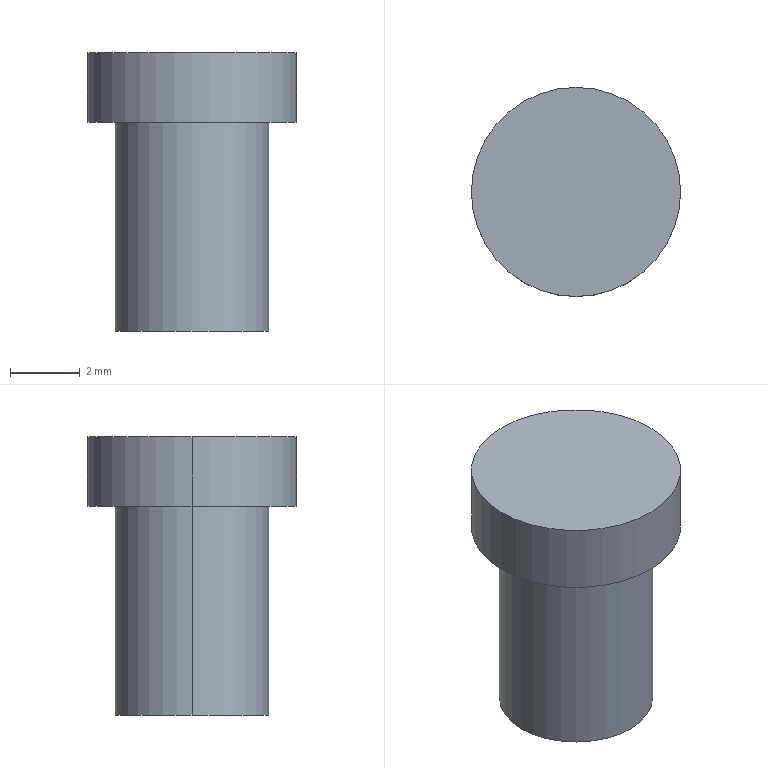Part | SolidWorks | features Extrusion 1, ICE 1 | 1 solid | 7 faces | box 6 x 6 x 8 mm | volume 147.781 mm3 | cylinder 4 | plane 3 | commonest cylinder face diameters 4.4 x2 6 x2
STEP:
#1=CARTESIAN_POINT('',(3.,0.,2.));
#2=VERTEX_POINT('',#1);
#3=CARTESIAN_POINT('',(-3.,0.,2.));
#4=VERTEX_POINT('',#3);
#5=CARTESIAN_POINT('',(0.,0.,2.));
#6=DIRECTION('',(0.,0.,1.));
#7=DIRECTION('',(1.,0.,0.));
#8=AXIS2_PLACEMENT_3D('',#5,#6,#7);
#9=CIRCLE('',#8,3.);
#10=EDGE_CURVE('',#2,#4,#9,.T.);
#11=ORIENTED_EDGE('',*,*,#10,.F.);
#12=CARTESIAN_POINT('',(3.,0.,0.));
#13=VERTEX_POINT('',#12);
#14=CARTESIAN_POINT('',(3.,0.,2.));
#15=DIRECTION('',(0.,0.,-1.));
#16=VECTOR('',#15,1000.);
#17=LINE('',#14,#16);
#18=EDGE_CURVE('',#2,#13,#17,.T.);
#19=ORIENTED_EDGE('',*,*,#18,.T.);
#20=CARTESIAN_POINT('',(-3.,0.,0.));
#21=VERTEX_POINT('',#20);
#22=CARTESIAN_POINT('',(0.,0.,0.));
#23=DIRECTION('',(0.,0.,1.));
#24=DIRECTION('',(1.,0.,0.));
#25=AXIS2_PLACEMENT_3D('',#22,#23,#24);
#26=CIRCLE('',#25,3.);
#27=EDGE_CURVE('',#13,#21,#26,.T.);
#28=ORIENTED_EDGE('',*,*,#27,.T.);
#29=CARTESIAN_POINT('',(-3.,0.,2.));
#30=DIRECTION('',(0.,0.,-1.));
#31=VECTOR('',#30,1000.);
#32=LINE('',#29,#31);
#33=EDGE_CURVE('',#4,#21,#32,.T.);
#34=ORIENTED_EDGE('',*,*,#33,.F.);
#35=EDGE_LOOP('',(#11,#19,#28,#34));
#36=FACE_OUTER_BOUND('',#35,.T.);
#37=CARTESIAN_POINT('',(0.,0.,2.));
#38=DIRECTION('',(0.,0.,-1.));
#39=DIRECTION('',(-1.,0.,0.));
#40=AXIS2_PLACEMENT_3D('',#37,#38,#39);
#41=CYLINDRICAL_SURFACE('',#40,3.);
#42=ADVANCED_FACE('',(#36),#41,.T.);
#43=CARTESIAN_POINT('',(2.2,0.,-6.));
#44=VERTEX_POINT('',#43);
#45=CARTESIAN_POINT('',(-2.2,0.,-6.));
#46=VERTEX_POINT('',#45);
#47=CARTESIAN_POINT('',(0.,0.,-6.));
#48=DIRECTION('',(0.,0.,1.));
#49=DIRECTION('',(1.,0.,0.));
#50=AXIS2_PLACEMENT_3D('',#47,#48,#49);
#51=CIRCLE('',#50,2.2);
#52=EDGE_CURVE('',#44,#46,#51,.T.);
#53=ORIENTED_EDGE('',*,*,#52,.T.);
#54=CARTESIAN_POINT('',(-2.2,0.,0.));
#55=VERTEX_POINT('',#54);
#56=CARTESIAN_POINT('',(-2.2,0.,-6.));
#57=DIRECTION('',(0.,0.,1.));
#58=VECTOR('',#57,1000.);
#59=LINE('',#56,#58);
#60=EDGE_CURVE('',#46,#55,#59,.T.);
#61=ORIENTED_EDGE('',*,*,#60,.T.);
#62=CARTESIAN_POINT('',(2.2,0.,0.));
#63=VERTEX_POINT('',#62);
#64=CARTESIAN_POINT('',(0.,0.,0.));
#65=DIRECTION('',(0.,0.,1.));
#66=DIRECTION('',(1.,0.,0.));
#67=AXIS2_PLACEMENT_3D('',#64,#65,#66);
#68=CIRCLE('',#67,2.2);
#69=EDGE_CURVE('',#63,#55,#68,.T.);
#70=ORIENTED_EDGE('',*,*,#69,.F.);
#71=CARTESIAN_POINT('',(2.2,0.,-6.));
#72=DIRECTION('',(0.,0.,1.));
#73=VECTOR('',#72,1000.);
#74=LINE('',#71,#73);
#75=EDGE_CURVE('',#44,#63,#74,.T.);
#76=ORIENTED_EDGE('',*,*,#75,.F.);
#77=EDGE_LOOP('',(#53,#61,#70,#76));
#78=FACE_OUTER_BOUND('',#77,.T.);
#79=CARTESIAN_POINT('',(0.,0.,-6.));
#80=DIRECTION('',(0.,0.,1.));
#81=DIRECTION('',(1.,0.,0.));
#82=AXIS2_PLACEMENT_3D('',#79,#80,#81);
#83=CYLINDRICAL_SURFACE('',#82,2.2);
#84=ADVANCED_FACE('',(#78),#83,.T.);
#85=ORIENTED_EDGE('',*,*,#60,.F.);
#86=CARTESIAN_POINT('',(0.,0.,-6.));
#87=DIRECTION('',(0.,0.,1.));
#88=DIRECTION('',(1.,0.,0.));
#89=AXIS2_PLACEMENT_3D('',#86,#87,#88);
#90=CIRCLE('',#89,2.2);
#91=EDGE_CURVE('',#46,#44,#90,.T.);
#92=ORIENTED_EDGE('',*,*,#91,.T.);
#93=ORIENTED_EDGE('',*,*,#75,.T.);
#94=CARTESIAN_POINT('',(0.,0.,0.));
#95=DIRECTION('',(0.,0.,1.));
#96=DIRECTION('',(1.,0.,0.));
#97=AXIS2_PLACEMENT_3D('',#94,#95,#96);
#98=CIRCLE('',#97,2.2);
#99=EDGE_CURVE('',#55,#63,#98,.T.);
#100=ORIENTED_EDGE('',*,*,#99,.F.);
#101=EDGE_LOOP('',(#85,#92,#93,#100));
#102=FACE_OUTER_BOUND('',#101,.T.);
#103=CARTESIAN_POINT('',(0.,0.,-6.));
#104=DIRECTION('',(0.,0.,1.));
#105=DIRECTION('',(1.,0.,0.));
#106=AXIS2_PLACEMENT_3D('',#103,#104,#105);
#107=CYLINDRICAL_SURFACE('',#106,2.2);
#108=ADVANCED_FACE('',(#102),#107,.T.);
#109=ORIENTED_EDGE('',*,*,#52,.F.);
#110=ORIENTED_EDGE('',*,*,#91,.F.);
#111=EDGE_LOOP('',(#109,#110));
#112=FACE_OUTER_BOUND('',#111,.T.);
#113=CARTESIAN_POINT('',(0.,0.,-6.));
#114=DIRECTION('',(0.,0.,1.));
#115=DIRECTION('',(1.,0.,0.));
#116=AXIS2_PLACEMENT_3D('',#113,#114,#115);
#117=PLANE('',#116);
#118=ADVANCED_FACE('',(#112),#117,.F.);
#119=ORIENTED_EDGE('',*,*,#18,.F.);
#120=CARTESIAN_POINT('',(0.,0.,2.));
#121=DIRECTION('',(0.,0.,1.));
#122=DIRECTION('',(1.,0.,0.));
#123=AXIS2_PLACEMENT_3D('',#120,#121,#122);
#124=CIRCLE('',#123,3.);
#125=EDGE_CURVE('',#4,#2,#124,.T.);
#126=ORIENTED_EDGE('',*,*,#125,.F.);
#127=ORIENTED_EDGE('',*,*,#33,.T.);
#128=CARTESIAN_POINT('',(0.,0.,0.));
#129=DIRECTION('',(0.,0.,1.));
#130=DIRECTION('',(1.,0.,0.));
#131=AXIS2_PLACEMENT_3D('',#128,#129,#130);
#132=CIRCLE('',#131,3.);
#133=EDGE_CURVE('',#21,#13,#132,.T.);
#134=ORIENTED_EDGE('',*,*,#133,.T.);
#135=EDGE_LOOP('',(#119,#126,#127,#134));
#136=FACE_OUTER_BOUND('',#135,.T.);
#137=CARTESIAN_POINT('',(0.,0.,2.));
#138=DIRECTION('',(0.,0.,-1.));
#139=DIRECTION('',(-1.,0.,0.));
#140=AXIS2_PLACEMENT_3D('',#137,#138,#139);
#141=CYLINDRICAL_SURFACE('',#140,3.);
#142=ADVANCED_FACE('',(#136),#141,.T.);
#143=ORIENTED_EDGE('',*,*,#125,.T.);
#144=ORIENTED_EDGE('',*,*,#10,.T.);
#145=EDGE_LOOP('',(#143,#144));
#146=FACE_OUTER_BOUND('',#145,.T.);
#147=CARTESIAN_POINT('',(0.,0.,2.));
#148=DIRECTION('',(0.,0.,1.));
#149=DIRECTION('',(1.,0.,0.));
#150=AXIS2_PLACEMENT_3D('',#147,#148,#149);
#151=PLANE('',#150);
#152=ADVANCED_FACE('',(#146),#151,.T.);
#153=ORIENTED_EDGE('',*,*,#69,.T.);
#154=ORIENTED_EDGE('',*,*,#99,.T.);
#155=EDGE_LOOP('',(#153,#154));
#156=FACE_BOUND('',#155,.T.);
#157=ORIENTED_EDGE('',*,*,#133,.F.);
#158=ORIENTED_EDGE('',*,*,#27,.F.);
#159=EDGE_LOOP('',(#157,#158));
#160=FACE_OUTER_BOUND('',#159,.T.);
#161=CARTESIAN_POINT('',(0.,0.,0.));
#162=DIRECTION('',(0.,0.,1.));
#163=DIRECTION('',(1.,0.,0.));
#164=AXIS2_PLACEMENT_3D('',#161,#162,#163);
#165=PLANE('',#164);
#166=ADVANCED_FACE('',(#156,#160),#165,.F.);
#167=CLOSED_SHELL('',(#42,#84,#108,#118,#142,#152,#166));
#168=MANIFOLD_SOLID_BREP('',#167);
#169=CARTESIAN_POINT('',(0.,0.,0.));
#170=DIRECTION('',(0.,0.,1.));
#171=DIRECTION('',(1.,0.,0.));
#172=AXIS2_PLACEMENT_3D('',#169,#170,#171);
#173=(LENGTH_UNIT()NAMED_UNIT(*)SI_UNIT(.MILLI.,.METRE.));
#174=UNCERTAINTY_MEASURE_WITH_UNIT(LENGTH_MEASURE(0.00001),#173,'','');
#175=(NAMED_UNIT(*)PLANE_ANGLE_UNIT()SI_UNIT($,.RADIAN.));
#176=(NAMED_UNIT(*)SI_UNIT($,.STERADIAN.)SOLID_ANGLE_UNIT());
#177=(GEOMETRIC_REPRESENTATION_CONTEXT(3)GLOBAL_UNCERTAINTY_ASSIGNED_CONTEXT((#174))GLOBAL_UNIT_ASSIGNED_CONTEXT((#173,#175,#176))REPRESENTATION_CONTEXT('',''));
#178=ADVANCED_BREP_SHAPE_REPRESENTATION('',(#168,#172),#177);